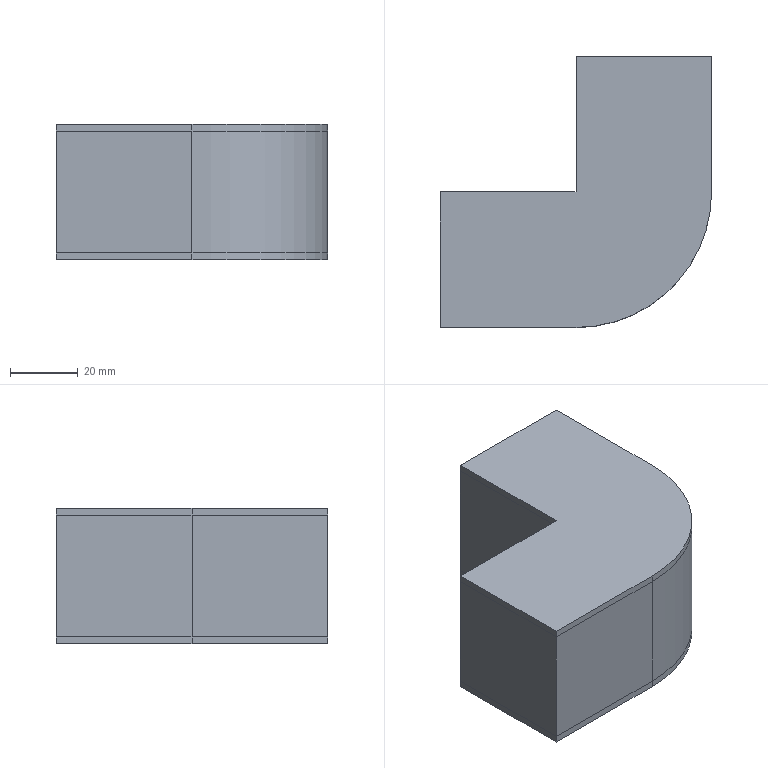Part | 3 solids | 34 faces | box 80 x 80 x 40 mm | volume 39085 mm3 | plane 30 | cylinder 4 | commonest cylinder face diameters 80 x3 76 x1
STEP:
#1=CARTESIAN_POINT('',(-40.,0.,38.));
#2=VERTEX_POINT('',#1);
#3=CARTESIAN_POINT('',(0.,0.,38.));
#4=VERTEX_POINT('',#3);
#5=CARTESIAN_POINT('',(-40.,0.,38.));
#6=DIRECTION('',(1.,0.,0.));
#7=VECTOR('',#6,1000.);
#8=LINE('',#5,#7);
#9=EDGE_CURVE('',#2,#4,#8,.T.);
#10=ORIENTED_EDGE('',*,*,#9,.F.);
#11=CARTESIAN_POINT('',(-40.,0.,40.));
#12=VERTEX_POINT('',#11);
#13=CARTESIAN_POINT('',(-40.,0.,40.));
#14=DIRECTION('',(0.,0.,-1.));
#15=VECTOR('',#14,1000.);
#16=LINE('',#13,#15);
#17=EDGE_CURVE('',#12,#2,#16,.T.);
#18=ORIENTED_EDGE('',*,*,#17,.F.);
#19=CARTESIAN_POINT('',(0.,0.,40.));
#20=VERTEX_POINT('',#19);
#21=CARTESIAN_POINT('',(-40.,0.,40.));
#22=DIRECTION('',(-1.,0.,0.));
#23=VECTOR('',#22,1000.);
#24=LINE('',#21,#23);
#25=EDGE_CURVE('',#20,#12,#24,.T.);
#26=ORIENTED_EDGE('',*,*,#25,.F.);
#27=CARTESIAN_POINT('',(0.,0.,40.));
#28=DIRECTION('',(0.,0.,-1.));
#29=VECTOR('',#28,1000.);
#30=LINE('',#27,#29);
#31=EDGE_CURVE('',#20,#4,#30,.T.);
#32=ORIENTED_EDGE('',*,*,#31,.T.);
#33=EDGE_LOOP('',(#10,#18,#26,#32));
#34=FACE_OUTER_BOUND('',#33,.T.);
#35=CARTESIAN_POINT('',(-40.,0.,40.));
#36=DIRECTION('',(0.,-1.,0.));
#37=DIRECTION('',(0.,0.,-1.));
#38=AXIS2_PLACEMENT_3D('',#35,#36,#37);
#39=PLANE('',#38);
#40=ADVANCED_FACE('',(#34),#39,.F.);
#41=CARTESIAN_POINT('',(-40.,-40.,38.));
#42=VERTEX_POINT('',#41);
#43=CARTESIAN_POINT('',(-40.,-40.,38.));
#44=DIRECTION('',(0.,1.,0.));
#45=VECTOR('',#44,1000.);
#46=LINE('',#43,#45);
#47=EDGE_CURVE('',#42,#2,#46,.T.);
#48=ORIENTED_EDGE('',*,*,#47,.F.);
#49=CARTESIAN_POINT('',(-40.,-40.,40.));
#50=VERTEX_POINT('',#49);
#51=CARTESIAN_POINT('',(-40.,-40.,40.));
#52=DIRECTION('',(0.,0.,-1.));
#53=VECTOR('',#52,1000.);
#54=LINE('',#51,#53);
#55=EDGE_CURVE('',#50,#42,#54,.T.);
#56=ORIENTED_EDGE('',*,*,#55,.F.);
#57=CARTESIAN_POINT('',(-40.,-40.,40.));
#58=DIRECTION('',(0.,-1.,0.));
#59=VECTOR('',#58,1000.);
#60=LINE('',#57,#59);
#61=EDGE_CURVE('',#12,#50,#60,.T.);
#62=ORIENTED_EDGE('',*,*,#61,.F.);
#63=ORIENTED_EDGE('',*,*,#17,.T.);
#64=EDGE_LOOP('',(#48,#56,#62,#63));
#65=FACE_OUTER_BOUND('',#64,.T.);
#66=CARTESIAN_POINT('',(-40.,-40.,40.));
#67=DIRECTION('',(1.,0.,0.));
#68=DIRECTION('',(0.,0.,-1.));
#69=AXIS2_PLACEMENT_3D('',#66,#67,#68);
#70=PLANE('',#69);
#71=ADVANCED_FACE('',(#65),#70,.F.);
#72=CARTESIAN_POINT('',(0.,-40.,38.));
#73=VERTEX_POINT('',#72);
#74=CARTESIAN_POINT('',(0.,-40.,38.));
#75=DIRECTION('',(-1.,0.,0.));
#76=VECTOR('',#75,1000.);
#77=LINE('',#74,#76);
#78=EDGE_CURVE('',#73,#42,#77,.T.);
#79=ORIENTED_EDGE('',*,*,#78,.F.);
#80=CARTESIAN_POINT('',(0.,-40.,40.));
#81=VERTEX_POINT('',#80);
#82=CARTESIAN_POINT('',(0.,-40.,40.));
#83=DIRECTION('',(0.,0.,-1.));
#84=VECTOR('',#83,1000.);
#85=LINE('',#82,#84);
#86=EDGE_CURVE('',#81,#73,#85,.T.);
#87=ORIENTED_EDGE('',*,*,#86,.F.);
#88=CARTESIAN_POINT('',(0.,-40.,40.));
#89=DIRECTION('',(1.,0.,0.));
#90=VECTOR('',#89,1000.);
#91=LINE('',#88,#90);
#92=EDGE_CURVE('',#50,#81,#91,.T.);
#93=ORIENTED_EDGE('',*,*,#92,.F.);
#94=ORIENTED_EDGE('',*,*,#55,.T.);
#95=EDGE_LOOP('',(#79,#87,#93,#94));
#96=FACE_OUTER_BOUND('',#95,.T.);
#97=CARTESIAN_POINT('',(0.,-40.,40.));
#98=DIRECTION('',(0.,1.,0.));
#99=DIRECTION('',(0.,0.,1.));
#100=AXIS2_PLACEMENT_3D('',#97,#98,#99);
#101=PLANE('',#100);
#102=ADVANCED_FACE('',(#96),#101,.F.);
#103=CARTESIAN_POINT('',(40.,0.,38.));
#104=VERTEX_POINT('',#103);
#105=CARTESIAN_POINT('',(0.,0.,38.));
#106=DIRECTION('',(0.,0.,-1.));
#107=DIRECTION('',(-1.,0.,0.));
#108=AXIS2_PLACEMENT_3D('',#105,#106,#107);
#109=CIRCLE('',#108,40.);
#110=EDGE_CURVE('',#104,#73,#109,.T.);
#111=ORIENTED_EDGE('',*,*,#110,.F.);
#112=CARTESIAN_POINT('',(40.,0.,40.));
#113=VERTEX_POINT('',#112);
#114=CARTESIAN_POINT('',(40.,0.,40.));
#115=DIRECTION('',(0.,0.,-1.));
#116=VECTOR('',#115,1000.);
#117=LINE('',#114,#116);
#118=EDGE_CURVE('',#113,#104,#117,.T.);
#119=ORIENTED_EDGE('',*,*,#118,.F.);
#120=CARTESIAN_POINT('',(0.,0.,40.));
#121=DIRECTION('',(0.,0.,1.));
#122=DIRECTION('',(1.,0.,0.));
#123=AXIS2_PLACEMENT_3D('',#120,#121,#122);
#124=CIRCLE('',#123,40.);
#125=EDGE_CURVE('',#81,#113,#124,.T.);
#126=ORIENTED_EDGE('',*,*,#125,.F.);
#127=ORIENTED_EDGE('',*,*,#86,.T.);
#128=EDGE_LOOP('',(#111,#119,#126,#127));
#129=FACE_OUTER_BOUND('',#128,.T.);
#130=CARTESIAN_POINT('',(0.,0.,40.));
#131=DIRECTION('',(0.,0.,-1.));
#132=DIRECTION('',(-1.,0.,0.));
#133=AXIS2_PLACEMENT_3D('',#130,#131,#132);
#134=CYLINDRICAL_SURFACE('',#133,40.);
#135=ADVANCED_FACE('',(#129),#134,.T.);
#136=CARTESIAN_POINT('',(40.,40.,38.));
#137=VERTEX_POINT('',#136);
#138=CARTESIAN_POINT('',(40.,0.,38.));
#139=DIRECTION('',(0.,-1.,0.));
#140=VECTOR('',#139,1000.);
#141=LINE('',#138,#140);
#142=EDGE_CURVE('',#137,#104,#141,.T.);
#143=ORIENTED_EDGE('',*,*,#142,.F.);
#144=CARTESIAN_POINT('',(40.,40.,40.));
#145=VERTEX_POINT('',#144);
#146=CARTESIAN_POINT('',(40.,40.,40.));
#147=DIRECTION('',(0.,0.,-1.));
#148=VECTOR('',#147,1000.);
#149=LINE('',#146,#148);
#150=EDGE_CURVE('',#145,#137,#149,.T.);
#151=ORIENTED_EDGE('',*,*,#150,.F.);
#152=CARTESIAN_POINT('',(40.,0.,40.));
#153=DIRECTION('',(0.,1.,0.));
#154=VECTOR('',#153,1000.);
#155=LINE('',#152,#154);
#156=EDGE_CURVE('',#113,#145,#155,.T.);
#157=ORIENTED_EDGE('',*,*,#156,.F.);
#158=ORIENTED_EDGE('',*,*,#118,.T.);
#159=EDGE_LOOP('',(#143,#151,#157,#158));
#160=FACE_OUTER_BOUND('',#159,.T.);
#161=CARTESIAN_POINT('',(40.,0.,40.));
#162=DIRECTION('',(-1.,0.,0.));
#163=DIRECTION('',(0.,0.,1.));
#164=AXIS2_PLACEMENT_3D('',#161,#162,#163);
#165=PLANE('',#164);
#166=ADVANCED_FACE('',(#160),#165,.F.);
#167=CARTESIAN_POINT('',(0.,40.,38.));
#168=VERTEX_POINT('',#167);
#169=CARTESIAN_POINT('',(0.,40.,38.));
#170=DIRECTION('',(1.,0.,0.));
#171=VECTOR('',#170,1000.);
#172=LINE('',#169,#171);
#173=EDGE_CURVE('',#168,#137,#172,.T.);
#174=ORIENTED_EDGE('',*,*,#173,.F.);
#175=CARTESIAN_POINT('',(0.,40.,40.));
#176=VERTEX_POINT('',#175);
#177=CARTESIAN_POINT('',(0.,40.,40.));
#178=DIRECTION('',(0.,0.,-1.));
#179=VECTOR('',#178,1000.);
#180=LINE('',#177,#179);
#181=EDGE_CURVE('',#176,#168,#180,.T.);
#182=ORIENTED_EDGE('',*,*,#181,.F.);
#183=CARTESIAN_POINT('',(0.,40.,40.));
#184=DIRECTION('',(-1.,0.,0.));
#185=VECTOR('',#184,1000.);
#186=LINE('',#183,#185);
#187=EDGE_CURVE('',#145,#176,#186,.T.);
#188=ORIENTED_EDGE('',*,*,#187,.F.);
#189=ORIENTED_EDGE('',*,*,#150,.T.);
#190=EDGE_LOOP('',(#174,#182,#188,#189));
#191=FACE_OUTER_BOUND('',#190,.T.);
#192=CARTESIAN_POINT('',(0.,40.,40.));
#193=DIRECTION('',(0.,-1.,0.));
#194=DIRECTION('',(0.,0.,-1.));
#195=AXIS2_PLACEMENT_3D('',#192,#193,#194);
#196=PLANE('',#195);
#197=ADVANCED_FACE('',(#191),#196,.F.);
#198=CARTESIAN_POINT('',(0.,0.,38.));
#199=DIRECTION('',(0.,1.,0.));
#200=VECTOR('',#199,1000.);
#201=LINE('',#198,#200);
#202=EDGE_CURVE('',#4,#168,#201,.T.);
#203=ORIENTED_EDGE('',*,*,#202,.F.);
#204=ORIENTED_EDGE('',*,*,#31,.F.);
#205=CARTESIAN_POINT('',(0.,0.,40.));
#206=DIRECTION('',(0.,-1.,0.));
#207=VECTOR('',#206,1000.);
#208=LINE('',#205,#207);
#209=EDGE_CURVE('',#176,#20,#208,.T.);
#210=ORIENTED_EDGE('',*,*,#209,.F.);
#211=ORIENTED_EDGE('',*,*,#181,.T.);
#212=EDGE_LOOP('',(#203,#204,#210,#211));
#213=FACE_OUTER_BOUND('',#212,.T.);
#214=CARTESIAN_POINT('',(0.,0.,40.));
#215=DIRECTION('',(1.,0.,0.));
#216=DIRECTION('',(0.,0.,-1.));
#217=AXIS2_PLACEMENT_3D('',#214,#215,#216);
#218=PLANE('',#217);
#219=ADVANCED_FACE('',(#213),#218,.F.);
#220=ORIENTED_EDGE('',*,*,#25,.T.);
#221=ORIENTED_EDGE('',*,*,#61,.T.);
#222=ORIENTED_EDGE('',*,*,#92,.T.);
#223=ORIENTED_EDGE('',*,*,#125,.T.);
#224=ORIENTED_EDGE('',*,*,#156,.T.);
#225=ORIENTED_EDGE('',*,*,#187,.T.);
#226=ORIENTED_EDGE('',*,*,#209,.T.);
#227=EDGE_LOOP('',(#220,#221,#222,#223,#224,#225,#226));
#228=FACE_OUTER_BOUND('',#227,.T.);
#229=CARTESIAN_POINT('',(0.,0.,40.));
#230=DIRECTION('',(0.,0.,1.));
#231=DIRECTION('',(1.,0.,0.));
#232=AXIS2_PLACEMENT_3D('',#229,#230,#231);
#233=PLANE('',#232);
#234=ADVANCED_FACE('',(#228),#233,.T.);
#235=ORIENTED_EDGE('',*,*,#47,.T.);
#236=ORIENTED_EDGE('',*,*,#9,.T.);
#237=ORIENTED_EDGE('',*,*,#202,.T.);
#238=ORIENTED_EDGE('',*,*,#173,.T.);
#239=ORIENTED_EDGE('',*,*,#142,.T.);
#240=ORIENTED_EDGE('',*,*,#110,.T.);
#241=ORIENTED_EDGE('',*,*,#78,.T.);
#242=EDGE_LOOP('',(#235,#236,#237,#238,#239,#240,#241));
#243=FACE_OUTER_BOUND('',#242,.T.);
#244=CARTESIAN_POINT('',(2.,38.,38.));
#245=DIRECTION('',(0.,0.,-1.));
#246=DIRECTION('',(-1.,0.,0.));
#247=AXIS2_PLACEMENT_3D('',#244,#245,#246);
#248=PLANE('',#247);
#249=ADVANCED_FACE('',(#243),#248,.T.);
#250=CLOSED_SHELL('',(#40,#71,#102,#135,#166,#197,#219,#234,#249));
#251=MANIFOLD_SOLID_BREP('',#250);
#252=CARTESIAN_POINT('',(-40.,-40.,2.));
#253=VERTEX_POINT('',#252);
#254=CARTESIAN_POINT('',(0.,-40.,2.));
#255=VERTEX_POINT('',#254);
#256=CARTESIAN_POINT('',(0.,-40.,2.));
#257=DIRECTION('',(1.,0.,0.));
#258=VECTOR('',#257,1000.);
#259=LINE('',#256,#258);
#260=EDGE_CURVE('',#253,#255,#259,.T.);
#261=ORIENTED_EDGE('',*,*,#260,.F.);
#262=CARTESIAN_POINT('',(-40.,-40.,0.));
#263=VERTEX_POINT('',#262);
#264=CARTESIAN_POINT('',(-40.,-40.,40.));
#265=DIRECTION('',(0.,0.,-1.));
#266=VECTOR('',#265,1000.);
#267=LINE('',#264,#266);
#268=EDGE_CURVE('',#253,#263,#267,.T.);
#269=ORIENTED_EDGE('',*,*,#268,.T.);
#270=CARTESIAN_POINT('',(0.,-40.,0.));
#271=VERTEX_POINT('',#270);
#272=CARTESIAN_POINT('',(0.,-40.,0.));
#273=DIRECTION('',(1.,0.,0.));
#274=VECTOR('',#273,1000.);
#275=LINE('',#272,#274);
#276=EDGE_CURVE('',#263,#271,#275,.T.);
#277=ORIENTED_EDGE('',*,*,#276,.T.);
#278=CARTESIAN_POINT('',(0.,-40.,40.));
#279=DIRECTION('',(0.,0.,-1.));
#280=VECTOR('',#279,1000.);
#281=LINE('',#278,#280);
#282=EDGE_CURVE('',#255,#271,#281,.T.);
#283=ORIENTED_EDGE('',*,*,#282,.F.);
#284=EDGE_LOOP('',(#261,#269,#277,#283));
#285=FACE_OUTER_BOUND('',#284,.T.);
#286=CARTESIAN_POINT('',(0.,-40.,40.));
#287=DIRECTION('',(0.,1.,0.));
#288=DIRECTION('',(0.,0.,1.));
#289=AXIS2_PLACEMENT_3D('',#286,#287,#288);
#290=PLANE('',#289);
#291=ADVANCED_FACE('',(#285),#290,.F.);
#292=CARTESIAN_POINT('',(40.,0.,2.));
#293=VERTEX_POINT('',#292);
#294=CARTESIAN_POINT('',(0.,0.,2.));
#295=DIRECTION('',(0.,0.,1.));
#296=DIRECTION('',(1.,0.,0.));
#297=AXIS2_PLACEMENT_3D('',#294,#295,#296);
#298=CIRCLE('',#297,40.);
#299=EDGE_CURVE('',#255,#293,#298,.T.);
#300=ORIENTED_EDGE('',*,*,#299,.F.);
#301=ORIENTED_EDGE('',*,*,#282,.T.);
#302=CARTESIAN_POINT('',(40.,0.,0.));
#303=VERTEX_POINT('',#302);
#304=CARTESIAN_POINT('',(0.,0.,0.));
#305=DIRECTION('',(0.,0.,1.));
#306=DIRECTION('',(1.,0.,0.));
#307=AXIS2_PLACEMENT_3D('',#304,#305,#306);
#308=CIRCLE('',#307,40.);
#309=EDGE_CURVE('',#271,#303,#308,.T.);
#310=ORIENTED_EDGE('',*,*,#309,.T.);
#311=CARTESIAN_POINT('',(40.,0.,40.));
#312=DIRECTION('',(0.,0.,-1.));
#313=VECTOR('',#312,1000.);
#314=LINE('',#311,#313);
#315=EDGE_CURVE('',#293,#303,#314,.T.);
#316=ORIENTED_EDGE('',*,*,#315,.F.);
#317=EDGE_LOOP('',(#300,#301,#310,#316));
#318=FACE_OUTER_BOUND('',#317,.T.);
#319=CARTESIAN_POINT('',(0.,0.,40.));
#320=DIRECTION('',(0.,0.,-1.));
#321=DIRECTION('',(-1.,0.,0.));
#322=AXIS2_PLACEMENT_3D('',#319,#320,#321);
#323=CYLINDRICAL_SURFACE('',#322,40.);
#324=ADVANCED_FACE('',(#318),#323,.T.);
#325=CARTESIAN_POINT('',(40.,40.,2.));
#326=VERTEX_POINT('',#325);
#327=CARTESIAN_POINT('',(40.,0.,2.));
#328=DIRECTION('',(0.,1.,0.));
#329=VECTOR('',#328,1000.);
#330=LINE('',#327,#329);
#331=EDGE_CURVE('',#293,#326,#330,.T.);
#332=ORIENTED_EDGE('',*,*,#331,.F.);
#333=ORIENTED_EDGE('',*,*,#315,.T.);
#334=CARTESIAN_POINT('',(40.,40.,0.));
#335=VERTEX_POINT('',#334);
#336=CARTESIAN_POINT('',(40.,0.,0.));
#337=DIRECTION('',(0.,1.,0.));
#338=VECTOR('',#337,1000.);
#339=LINE('',#336,#338);
#340=EDGE_CURVE('',#303,#335,#339,.T.);
#341=ORIENTED_EDGE('',*,*,#340,.T.);
#342=CARTESIAN_POINT('',(40.,40.,40.));
#343=DIRECTION('',(0.,0.,-1.));
#344=VECTOR('',#343,1000.);
#345=LINE('',#342,#344);
#346=EDGE_CURVE('',#326,#335,#345,.T.);
#347=ORIENTED_EDGE('',*,*,#346,.F.);
#348=EDGE_LOOP('',(#332,#333,#341,#347));
#349=FACE_OUTER_BOUND('',#348,.T.);
#350=CARTESIAN_POINT('',(40.,0.,40.));
#351=DIRECTION('',(-1.,0.,0.));
#352=DIRECTION('',(0.,0.,1.));
#353=AXIS2_PLACEMENT_3D('',#350,#351,#352);
#354=PLANE('',#353);
#355=ADVANCED_FACE('',(#349),#354,.F.);
#356=CARTESIAN_POINT('',(-40.,0.,2.));
#357=VERTEX_POINT('',#356);
#358=CARTESIAN_POINT('',(-40.,-40.,2.));
#359=DIRECTION('',(0.,-1.,0.));
#360=VECTOR('',#359,1000.);
#361=LINE('',#358,#360);
#362=EDGE_CURVE('',#357,#253,#361,.T.);
#363=ORIENTED_EDGE('',*,*,#362,.F.);
#364=CARTESIAN_POINT('',(-40.,0.,0.));
#365=VERTEX_POINT('',#364);
#366=CARTESIAN_POINT('',(-40.,0.,40.));
#367=DIRECTION('',(0.,0.,-1.));
#368=VECTOR('',#367,1000.);
#369=LINE('',#366,#368);
#370=EDGE_CURVE('',#357,#365,#369,.T.);
#371=ORIENTED_EDGE('',*,*,#370,.T.);
#372=CARTESIAN_POINT('',(-40.,-40.,0.));
#373=DIRECTION('',(0.,-1.,0.));
#374=VECTOR('',#373,1000.);
#375=LINE('',#372,#374);
#376=EDGE_CURVE('',#365,#263,#375,.T.);
#377=ORIENTED_EDGE('',*,*,#376,.T.);
#378=ORIENTED_EDGE('',*,*,#268,.F.);
#379=EDGE_LOOP('',(#363,#371,#377,#378));
#380=FACE_OUTER_BOUND('',#379,.T.);
#381=CARTESIAN_POINT('',(-40.,-40.,40.));
#382=DIRECTION('',(1.,0.,0.));
#383=DIRECTION('',(0.,0.,-1.));
#384=AXIS2_PLACEMENT_3D('',#381,#382,#383);
#385=PLANE('',#384);
#386=ADVANCED_FACE('',(#380),#385,.F.);
#387=CARTESIAN_POINT('',(0.,0.,2.));
#388=VERTEX_POINT('',#387);
#389=CARTESIAN_POINT('',(-40.,0.,2.));
#390=DIRECTION('',(-1.,0.,0.));
#391=VECTOR('',#390,1000.);
#392=LINE('',#389,#391);
#393=EDGE_CURVE('',#388,#357,#392,.T.);
#394=ORIENTED_EDGE('',*,*,#393,.F.);
#395=CARTESIAN_POINT('',(0.,0.,0.));
#396=VERTEX_POINT('',#395);
#397=CARTESIAN_POINT('',(0.,0.,40.));
#398=DIRECTION('',(0.,0.,-1.));
#399=VECTOR('',#398,1000.);
#400=LINE('',#397,#399);
#401=EDGE_CURVE('',#388,#396,#400,.T.);
#402=ORIENTED_EDGE('',*,*,#401,.T.);
#403=CARTESIAN_POINT('',(-40.,0.,0.));
#404=DIRECTION('',(-1.,0.,0.));
#405=VECTOR('',#404,1000.);
#406=LINE('',#403,#405);
#407=EDGE_CURVE('',#396,#365,#406,.T.);
#408=ORIENTED_EDGE('',*,*,#407,.T.);
#409=ORIENTED_EDGE('',*,*,#370,.F.);
#410=EDGE_LOOP('',(#394,#402,#408,#409));
#411=FACE_OUTER_BOUND('',#410,.T.);
#412=CARTESIAN_POINT('',(-40.,0.,40.));
#413=DIRECTION('',(0.,-1.,0.));
#414=DIRECTION('',(0.,0.,-1.));
#415=AXIS2_PLACEMENT_3D('',#412,#413,#414);
#416=PLANE('',#415);
#417=ADVANCED_FACE('',(#411),#416,.F.);
#418=ORIENTED_EDGE('',*,*,#407,.F.);
#419=CARTESIAN_POINT('',(0.,40.,0.));
#420=VERTEX_POINT('',#419);
#421=CARTESIAN_POINT('',(0.,0.,0.));
#422=DIRECTION('',(0.,-1.,0.));
#423=VECTOR('',#422,1000.);
#424=LINE('',#421,#423);
#425=EDGE_CURVE('',#420,#396,#424,.T.);
#426=ORIENTED_EDGE('',*,*,#425,.F.);
#427=CARTESIAN_POINT('',(0.,40.,0.));
#428=DIRECTION('',(-1.,0.,0.));
#429=VECTOR('',#428,1000.);
#430=LINE('',#427,#429);
#431=EDGE_CURVE('',#335,#420,#430,.T.);
#432=ORIENTED_EDGE('',*,*,#431,.F.);
#433=ORIENTED_EDGE('',*,*,#340,.F.);
#434=ORIENTED_EDGE('',*,*,#309,.F.);
#435=ORIENTED_EDGE('',*,*,#276,.F.);
#436=ORIENTED_EDGE('',*,*,#376,.F.);
#437=EDGE_LOOP('',(#418,#426,#432,#433,#434,#435,#436));
#438=FACE_OUTER_BOUND('',#437,.T.);
#439=CARTESIAN_POINT('',(0.,0.,0.));
#440=DIRECTION('',(0.,0.,1.));
#441=DIRECTION('',(1.,0.,0.));
#442=AXIS2_PLACEMENT_3D('',#439,#440,#441);
#443=PLANE('',#442);
#444=ADVANCED_FACE('',(#438),#443,.F.);
#445=CARTESIAN_POINT('',(0.,40.,2.));
#446=VERTEX_POINT('',#445);
#447=CARTESIAN_POINT('',(0.,40.,2.));
#448=DIRECTION('',(-1.,0.,0.));
#449=VECTOR('',#448,1000.);
#450=LINE('',#447,#449);
#451=EDGE_CURVE('',#326,#446,#450,.T.);
#452=ORIENTED_EDGE('',*,*,#451,.F.);
#453=ORIENTED_EDGE('',*,*,#346,.T.);
#454=ORIENTED_EDGE('',*,*,#431,.T.);
#455=CARTESIAN_POINT('',(0.,40.,40.));
#456=DIRECTION('',(0.,0.,-1.));
#457=VECTOR('',#456,1000.);
#458=LINE('',#455,#457);
#459=EDGE_CURVE('',#446,#420,#458,.T.);
#460=ORIENTED_EDGE('',*,*,#459,.F.);
#461=EDGE_LOOP('',(#452,#453,#454,#460));
#462=FACE_OUTER_BOUND('',#461,.T.);
#463=CARTESIAN_POINT('',(0.,40.,40.));
#464=DIRECTION('',(0.,-1.,0.));
#465=DIRECTION('',(0.,0.,-1.));
#466=AXIS2_PLACEMENT_3D('',#463,#464,#465);
#467=PLANE('',#466);
#468=ADVANCED_FACE('',(#462),#467,.F.);
#469=CARTESIAN_POINT('',(0.,0.,2.));
#470=DIRECTION('',(0.,-1.,0.));
#471=VECTOR('',#470,1000.);
#472=LINE('',#469,#471);
#473=EDGE_CURVE('',#446,#388,#472,.T.);
#474=ORIENTED_EDGE('',*,*,#473,.F.);
#475=ORIENTED_EDGE('',*,*,#459,.T.);
#476=ORIENTED_EDGE('',*,*,#425,.T.);
#477=ORIENTED_EDGE('',*,*,#401,.F.);
#478=EDGE_LOOP('',(#474,#475,#476,#477));
#479=FACE_OUTER_BOUND('',#478,.T.);
#480=CARTESIAN_POINT('',(0.,0.,40.));
#481=DIRECTION('',(1.,0.,0.));
#482=DIRECTION('',(0.,0.,-1.));
#483=AXIS2_PLACEMENT_3D('',#480,#481,#482);
#484=PLANE('',#483);
#485=ADVANCED_FACE('',(#479),#484,.F.);
#486=ORIENTED_EDGE('',*,*,#393,.T.);
#487=ORIENTED_EDGE('',*,*,#362,.T.);
#488=ORIENTED_EDGE('',*,*,#260,.T.);
#489=ORIENTED_EDGE('',*,*,#299,.T.);
#490=ORIENTED_EDGE('',*,*,#331,.T.);
#491=ORIENTED_EDGE('',*,*,#451,.T.);
#492=ORIENTED_EDGE('',*,*,#473,.T.);
#493=EDGE_LOOP('',(#486,#487,#488,#489,#490,#491,#492));
#494=FACE_OUTER_BOUND('',#493,.T.);
#495=CARTESIAN_POINT('',(-38.,-2.,2.));
#496=DIRECTION('',(0.,0.,1.));
#497=DIRECTION('',(1.,0.,0.));
#498=AXIS2_PLACEMENT_3D('',#495,#496,#497);
#499=PLANE('',#498);
#500=ADVANCED_FACE('',(#494),#499,.T.);
#501=CLOSED_SHELL('',(#291,#324,#355,#386,#417,#444,#468,#485,#500));
#502=MANIFOLD_SOLID_BREP('',#501);
#503=CARTESIAN_POINT('',(0.,-38.,2.));
#504=VERTEX_POINT('',#503);
#505=CARTESIAN_POINT('',(38.,0.,2.));
#506=VERTEX_POINT('',#505);
#507=CARTESIAN_POINT('',(0.,0.,2.));
#508=DIRECTION('',(0.,0.,1.));
#509=DIRECTION('',(1.,0.,0.));
#510=AXIS2_PLACEMENT_3D('',#507,#508,#509);
#511=CIRCLE('',#510,38.);
#512=EDGE_CURVE('',#504,#506,#511,.T.);
#513=ORIENTED_EDGE('',*,*,#512,.T.);
#514=CARTESIAN_POINT('',(38.,38.,2.));
#515=VERTEX_POINT('',#514);
#516=CARTESIAN_POINT('',(38.,0.,2.));
#517=DIRECTION('',(0.,1.,0.));
#518=VECTOR('',#517,1000.);
#519=LINE('',#516,#518);
#520=EDGE_CURVE('',#506,#515,#519,.T.);
#521=ORIENTED_EDGE('',*,*,#520,.T.);
#522=CARTESIAN_POINT('',(2.,38.,2.));
#523=VERTEX_POINT('',#522);
#524=CARTESIAN_POINT('',(0.,38.,2.));
#525=DIRECTION('',(-1.,0.,0.));
#526=VECTOR('',#525,1000.);
#527=LINE('',#524,#526);
#528=EDGE_CURVE('',#515,#523,#527,.T.);
#529=ORIENTED_EDGE('',*,*,#528,.T.);
#530=CARTESIAN_POINT('',(2.,-2.,2.));
#531=VERTEX_POINT('',#530);
#532=CARTESIAN_POINT('',(2.,0.,2.));
#533=DIRECTION('',(0.,-1.,0.));
#534=VECTOR('',#533,1000.);
#535=LINE('',#532,#534);
#536=EDGE_CURVE('',#523,#531,#535,.T.);
#537=ORIENTED_EDGE('',*,*,#536,.T.);
#538=CARTESIAN_POINT('',(-38.,-2.,2.));
#539=VERTEX_POINT('',#538);
#540=CARTESIAN_POINT('',(-40.,-2.,2.));
#541=DIRECTION('',(-1.,0.,0.));
#542=VECTOR('',#541,1000.);
#543=LINE('',#540,#542);
#544=EDGE_CURVE('',#531,#539,#543,.T.);
#545=ORIENTED_EDGE('',*,*,#544,.T.);
#546=CARTESIAN_POINT('',(-38.,-38.,2.));
#547=VERTEX_POINT('',#546);
#548=CARTESIAN_POINT('',(-38.,-40.,2.));
#549=DIRECTION('',(0.,-1.,0.));
#550=VECTOR('',#549,1000.);
#551=LINE('',#548,#550);
#552=EDGE_CURVE('',#539,#547,#551,.T.);
#553=ORIENTED_EDGE('',*,*,#552,.T.);
#554=CARTESIAN_POINT('',(0.,-38.,2.));
#555=DIRECTION('',(1.,0.,0.));
#556=VECTOR('',#555,1000.);
#557=LINE('',#554,#556);
#558=EDGE_CURVE('',#547,#504,#557,.T.);
#559=ORIENTED_EDGE('',*,*,#558,.T.);
#560=EDGE_LOOP('',(#513,#521,#529,#537,#545,#553,#559));
#561=FACE_BOUND('',#560,.T.);
#562=CARTESIAN_POINT('',(0.,0.,2.));
#563=VERTEX_POINT('',#562);
#564=CARTESIAN_POINT('',(-40.,0.,2.));
#565=VERTEX_POINT('',#564);
#566=CARTESIAN_POINT('',(-40.,0.,2.));
#567=DIRECTION('',(-1.,0.,0.));
#568=VECTOR('',#567,1000.);
#569=LINE('',#566,#568);
#570=EDGE_CURVE('',#563,#565,#569,.T.);
#571=ORIENTED_EDGE('',*,*,#570,.F.);
#572=CARTESIAN_POINT('',(0.,40.,2.));
#573=VERTEX_POINT('',#572);
#574=CARTESIAN_POINT('',(0.,0.,2.));
#575=DIRECTION('',(0.,-1.,0.));
#576=VECTOR('',#575,1000.);
#577=LINE('',#574,#576);
#578=EDGE_CURVE('',#573,#563,#577,.T.);
#579=ORIENTED_EDGE('',*,*,#578,.F.);
#580=CARTESIAN_POINT('',(40.,40.,2.));
#581=VERTEX_POINT('',#580);
#582=CARTESIAN_POINT('',(0.,40.,2.));
#583=DIRECTION('',(-1.,0.,0.));
#584=VECTOR('',#583,1000.);
#585=LINE('',#582,#584);
#586=EDGE_CURVE('',#581,#573,#585,.T.);
#587=ORIENTED_EDGE('',*,*,#586,.F.);
#588=CARTESIAN_POINT('',(40.,0.,2.));
#589=VERTEX_POINT('',#588);
#590=CARTESIAN_POINT('',(40.,0.,2.));
#591=DIRECTION('',(0.,1.,0.));
#592=VECTOR('',#591,1000.);
#593=LINE('',#590,#592);
#594=EDGE_CURVE('',#589,#581,#593,.T.);
#595=ORIENTED_EDGE('',*,*,#594,.F.);
#596=CARTESIAN_POINT('',(0.,-40.,2.));
#597=VERTEX_POINT('',#596);
#598=CARTESIAN_POINT('',(0.,0.,2.));
#599=DIRECTION('',(0.,0.,1.));
#600=DIRECTION('',(1.,0.,0.));
#601=AXIS2_PLACEMENT_3D('',#598,#599,#600);
#602=CIRCLE('',#601,40.);
#603=EDGE_CURVE('',#597,#589,#602,.T.);
#604=ORIENTED_EDGE('',*,*,#603,.F.);
#605=CARTESIAN_POINT('',(-40.,-40.,2.));
#606=VERTEX_POINT('',#605);
#607=CARTESIAN_POINT('',(0.,-40.,2.));
#608=DIRECTION('',(1.,0.,0.));
#609=VECTOR('',#608,1000.);
#610=LINE('',#607,#609);
#611=EDGE_CURVE('',#606,#597,#610,.T.);
#612=ORIENTED_EDGE('',*,*,#611,.F.);
#613=CARTESIAN_POINT('',(-40.,-40.,2.));
#614=DIRECTION('',(0.,-1.,0.));
#615=VECTOR('',#614,1000.);
#616=LINE('',#613,#615);
#617=EDGE_CURVE('',#565,#606,#616,.T.);
#618=ORIENTED_EDGE('',*,*,#617,.F.);
#619=EDGE_LOOP('',(#571,#579,#587,#595,#604,#612,#618));
#620=FACE_OUTER_BOUND('',#619,.T.);
#621=CARTESIAN_POINT('',(-38.,-2.,2.));
#622=DIRECTION('',(0.,0.,1.));
#623=DIRECTION('',(1.,0.,0.));
#624=AXIS2_PLACEMENT_3D('',#621,#622,#623);
#625=PLANE('',#624);
#626=ADVANCED_FACE('',(#561,#620),#625,.F.);
#627=CARTESIAN_POINT('',(2.,-2.,38.));
#628=VERTEX_POINT('',#627);
#629=CARTESIAN_POINT('',(2.,-2.,40.));
#630=DIRECTION('',(0.,0.,-1.));
#631=VECTOR('',#630,1000.);
#632=LINE('',#629,#631);
#633=EDGE_CURVE('',#628,#531,#632,.T.);
#634=ORIENTED_EDGE('',*,*,#633,.F.);
#635=CARTESIAN_POINT('',(-38.,-2.,38.));
#636=VERTEX_POINT('',#635);
#637=CARTESIAN_POINT('',(2.,-2.,38.));
#638=DIRECTION('',(-1.,0.,0.));
#639=VECTOR('',#638,1000.);
#640=LINE('',#637,#639);
#641=EDGE_CURVE('',#628,#636,#640,.T.);
#642=ORIENTED_EDGE('',*,*,#641,.T.);
#643=CARTESIAN_POINT('',(-38.,-2.,40.));
#644=DIRECTION('',(0.,0.,-1.));
#645=VECTOR('',#644,1000.);
#646=LINE('',#643,#645);
#647=EDGE_CURVE('',#636,#539,#646,.T.);
#648=ORIENTED_EDGE('',*,*,#647,.T.);
#649=ORIENTED_EDGE('',*,*,#544,.F.);
#650=EDGE_LOOP('',(#634,#642,#648,#649));
#651=FACE_OUTER_BOUND('',#650,.T.);
#652=CARTESIAN_POINT('',(-40.,-2.,40.));
#653=DIRECTION('',(0.,-1.,0.));
#654=DIRECTION('',(0.,0.,-1.));
#655=AXIS2_PLACEMENT_3D('',#652,#653,#654);
#656=PLANE('',#655);
#657=ADVANCED_FACE('',(#651),#656,.T.);
#658=CARTESIAN_POINT('',(2.,38.,38.));
#659=VERTEX_POINT('',#658);
#660=CARTESIAN_POINT('',(2.,38.,40.));
#661=DIRECTION('',(0.,0.,-1.));
#662=VECTOR('',#661,1000.);
#663=LINE('',#660,#662);
#664=EDGE_CURVE('',#659,#523,#663,.T.);
#665=ORIENTED_EDGE('',*,*,#664,.F.);
#666=CARTESIAN_POINT('',(2.,38.,38.));
#667=DIRECTION('',(0.,-1.,0.));
#668=VECTOR('',#667,1000.);
#669=LINE('',#666,#668);
#670=EDGE_CURVE('',#659,#628,#669,.T.);
#671=ORIENTED_EDGE('',*,*,#670,.T.);
#672=ORIENTED_EDGE('',*,*,#633,.T.);
#673=ORIENTED_EDGE('',*,*,#536,.F.);
#674=EDGE_LOOP('',(#665,#671,#672,#673));
#675=FACE_OUTER_BOUND('',#674,.T.);
#676=CARTESIAN_POINT('',(2.,0.,40.));
#677=DIRECTION('',(1.,0.,0.));
#678=DIRECTION('',(0.,0.,-1.));
#679=AXIS2_PLACEMENT_3D('',#676,#677,#678);
#680=PLANE('',#679);
#681=ADVANCED_FACE('',(#675),#680,.T.);
#682=CARTESIAN_POINT('',(0.,40.,38.));
#683=VERTEX_POINT('',#682);
#684=CARTESIAN_POINT('',(0.,40.,40.));
#685=DIRECTION('',(0.,0.,-1.));
#686=VECTOR('',#685,1000.);
#687=LINE('',#684,#686);
#688=EDGE_CURVE('',#683,#573,#687,.T.);
#689=ORIENTED_EDGE('',*,*,#688,.T.);
#690=ORIENTED_EDGE('',*,*,#578,.T.);
#691=CARTESIAN_POINT('',(0.,0.,38.));
#692=VERTEX_POINT('',#691);
#693=CARTESIAN_POINT('',(0.,0.,40.));
#694=DIRECTION('',(0.,0.,-1.));
#695=VECTOR('',#694,1000.);
#696=LINE('',#693,#695);
#697=EDGE_CURVE('',#692,#563,#696,.T.);
#698=ORIENTED_EDGE('',*,*,#697,.F.);
#699=CARTESIAN_POINT('',(0.,0.,38.));
#700=DIRECTION('',(0.,1.,0.));
#701=VECTOR('',#700,1000.);
#702=LINE('',#699,#701);
#703=EDGE_CURVE('',#692,#683,#702,.T.);
#704=ORIENTED_EDGE('',*,*,#703,.T.);
#705=EDGE_LOOP('',(#689,#690,#698,#704));
#706=FACE_OUTER_BOUND('',#705,.T.);
#707=CARTESIAN_POINT('',(0.,0.,40.));
#708=DIRECTION('',(1.,0.,0.));
#709=DIRECTION('',(0.,0.,-1.));
#710=AXIS2_PLACEMENT_3D('',#707,#708,#709);
#711=PLANE('',#710);
#712=ADVANCED_FACE('',(#706),#711,.F.);
#713=CARTESIAN_POINT('',(40.,40.,38.));
#714=VERTEX_POINT('',#713);
#715=CARTESIAN_POINT('',(40.,40.,40.));
#716=DIRECTION('',(0.,0.,-1.));
#717=VECTOR('',#716,1000.);
#718=LINE('',#715,#717);
#719=EDGE_CURVE('',#714,#581,#718,.T.);
#720=ORIENTED_EDGE('',*,*,#719,.T.);
#721=ORIENTED_EDGE('',*,*,#586,.T.);
#722=ORIENTED_EDGE('',*,*,#688,.F.);
#723=CARTESIAN_POINT('',(0.,40.,38.));
#724=DIRECTION('',(1.,0.,0.));
#725=VECTOR('',#724,1000.);
#726=LINE('',#723,#725);
#727=EDGE_CURVE('',#683,#714,#726,.T.);
#728=ORIENTED_EDGE('',*,*,#727,.T.);
#729=EDGE_LOOP('',(#720,#721,#722,#728));
#730=FACE_OUTER_BOUND('',#729,.T.);
#731=CARTESIAN_POINT('',(0.,40.,40.));
#732=DIRECTION('',(0.,-1.,0.));
#733=DIRECTION('',(0.,0.,-1.));
#734=AXIS2_PLACEMENT_3D('',#731,#732,#733);
#735=PLANE('',#734);
#736=ADVANCED_FACE('',(#730),#735,.F.);
#737=ORIENTED_EDGE('',*,*,#697,.T.);
#738=ORIENTED_EDGE('',*,*,#570,.T.);
#739=CARTESIAN_POINT('',(-40.,0.,38.));
#740=VERTEX_POINT('',#739);
#741=CARTESIAN_POINT('',(-40.,0.,40.));
#742=DIRECTION('',(0.,0.,-1.));
#743=VECTOR('',#742,1000.);
#744=LINE('',#741,#743);
#745=EDGE_CURVE('',#740,#565,#744,.T.);
#746=ORIENTED_EDGE('',*,*,#745,.F.);
#747=CARTESIAN_POINT('',(-40.,0.,38.));
#748=DIRECTION('',(1.,0.,0.));
#749=VECTOR('',#748,1000.);
#750=LINE('',#747,#749);
#751=EDGE_CURVE('',#740,#692,#750,.T.);
#752=ORIENTED_EDGE('',*,*,#751,.T.);
#753=EDGE_LOOP('',(#737,#738,#746,#752));
#754=FACE_OUTER_BOUND('',#753,.T.);
#755=CARTESIAN_POINT('',(-40.,0.,40.));
#756=DIRECTION('',(0.,-1.,0.));
#757=DIRECTION('',(0.,0.,-1.));
#758=AXIS2_PLACEMENT_3D('',#755,#756,#757);
#759=PLANE('',#758);
#760=ADVANCED_FACE('',(#754),#759,.F.);
#761=CARTESIAN_POINT('',(38.,38.,38.));
#762=VERTEX_POINT('',#761);
#763=CARTESIAN_POINT('',(38.,38.,38.));
#764=DIRECTION('',(-1.,0.,0.));
#765=VECTOR('',#764,1000.);
#766=LINE('',#763,#765);
#767=EDGE_CURVE('',#762,#659,#766,.T.);
#768=ORIENTED_EDGE('',*,*,#767,.F.);
#769=CARTESIAN_POINT('',(38.,0.,38.));
#770=VERTEX_POINT('',#769);
#771=CARTESIAN_POINT('',(38.,0.,38.));
#772=DIRECTION('',(0.,1.,0.));
#773=VECTOR('',#772,1000.);
#774=LINE('',#771,#773);
#775=EDGE_CURVE('',#770,#762,#774,.T.);
#776=ORIENTED_EDGE('',*,*,#775,.F.);
#777=CARTESIAN_POINT('',(0.,-38.,38.));
#778=VERTEX_POINT('',#777);
#779=CARTESIAN_POINT('',(0.,0.,38.));
#780=DIRECTION('',(0.,0.,1.));
#781=DIRECTION('',(1.,0.,0.));
#782=AXIS2_PLACEMENT_3D('',#779,#780,#781);
#783=CIRCLE('',#782,38.);
#784=EDGE_CURVE('',#778,#770,#783,.T.);
#785=ORIENTED_EDGE('',*,*,#784,.F.);
#786=CARTESIAN_POINT('',(-38.,-38.,38.));
#787=VERTEX_POINT('',#786);
#788=CARTESIAN_POINT('',(-38.,-38.,38.));
#789=DIRECTION('',(1.,0.,0.));
#790=VECTOR('',#789,1000.);
#791=LINE('',#788,#790);
#792=EDGE_CURVE('',#787,#778,#791,.T.);
#793=ORIENTED_EDGE('',*,*,#792,.F.);
#794=CARTESIAN_POINT('',(-38.,-2.,38.));
#795=DIRECTION('',(0.,-1.,0.));
#796=VECTOR('',#795,1000.);
#797=LINE('',#794,#796);
#798=EDGE_CURVE('',#636,#787,#797,.T.);
#799=ORIENTED_EDGE('',*,*,#798,.F.);
#800=ORIENTED_EDGE('',*,*,#641,.F.);
#801=ORIENTED_EDGE('',*,*,#670,.F.);
#802=EDGE_LOOP('',(#768,#776,#785,#793,#799,#800,#801));
#803=FACE_BOUND('',#802,.T.);
#804=CARTESIAN_POINT('',(-40.,-40.,38.));
#805=VERTEX_POINT('',#804);
#806=CARTESIAN_POINT('',(-40.,-40.,38.));
#807=DIRECTION('',(0.,1.,0.));
#808=VECTOR('',#807,1000.);
#809=LINE('',#806,#808);
#810=EDGE_CURVE('',#805,#740,#809,.T.);
#811=ORIENTED_EDGE('',*,*,#810,.F.);
#812=CARTESIAN_POINT('',(0.,-40.,38.));
#813=VERTEX_POINT('',#812);
#814=CARTESIAN_POINT('',(0.,-40.,38.));
#815=DIRECTION('',(-1.,0.,0.));
#816=VECTOR('',#815,1000.);
#817=LINE('',#814,#816);
#818=EDGE_CURVE('',#813,#805,#817,.T.);
#819=ORIENTED_EDGE('',*,*,#818,.F.);
#820=CARTESIAN_POINT('',(40.,0.,38.));
#821=VERTEX_POINT('',#820);
#822=CARTESIAN_POINT('',(0.,0.,38.));
#823=DIRECTION('',(0.,0.,-1.));
#824=DIRECTION('',(-1.,0.,0.));
#825=AXIS2_PLACEMENT_3D('',#822,#823,#824);
#826=CIRCLE('',#825,40.);
#827=EDGE_CURVE('',#821,#813,#826,.T.);
#828=ORIENTED_EDGE('',*,*,#827,.F.);
#829=CARTESIAN_POINT('',(40.,0.,38.));
#830=DIRECTION('',(0.,-1.,0.));
#831=VECTOR('',#830,1000.);
#832=LINE('',#829,#831);
#833=EDGE_CURVE('',#714,#821,#832,.T.);
#834=ORIENTED_EDGE('',*,*,#833,.F.);
#835=ORIENTED_EDGE('',*,*,#727,.F.);
#836=ORIENTED_EDGE('',*,*,#703,.F.);
#837=ORIENTED_EDGE('',*,*,#751,.F.);
#838=EDGE_LOOP('',(#811,#819,#828,#834,#835,#836,#837));
#839=FACE_OUTER_BOUND('',#838,.T.);
#840=CARTESIAN_POINT('',(2.,38.,38.));
#841=DIRECTION('',(0.,0.,-1.));
#842=DIRECTION('',(-1.,0.,0.));
#843=AXIS2_PLACEMENT_3D('',#840,#841,#842);
#844=PLANE('',#843);
#845=ADVANCED_FACE('',(#803,#839),#844,.F.);
#846=ORIENTED_EDGE('',*,*,#745,.T.);
#847=ORIENTED_EDGE('',*,*,#617,.T.);
#848=CARTESIAN_POINT('',(-40.,-40.,40.));
#849=DIRECTION('',(0.,0.,-1.));
#850=VECTOR('',#849,1000.);
#851=LINE('',#848,#850);
#852=EDGE_CURVE('',#805,#606,#851,.T.);
#853=ORIENTED_EDGE('',*,*,#852,.F.);
#854=ORIENTED_EDGE('',*,*,#810,.T.);
#855=EDGE_LOOP('',(#846,#847,#853,#854));
#856=FACE_OUTER_BOUND('',#855,.T.);
#857=CARTESIAN_POINT('',(-40.,-40.,40.));
#858=DIRECTION('',(1.,0.,0.));
#859=DIRECTION('',(0.,0.,-1.));
#860=AXIS2_PLACEMENT_3D('',#857,#858,#859);
#861=PLANE('',#860);
#862=ADVANCED_FACE('',(#856),#861,.F.);
#863=CARTESIAN_POINT('',(40.,0.,40.));
#864=DIRECTION('',(0.,0.,-1.));
#865=VECTOR('',#864,1000.);
#866=LINE('',#863,#865);
#867=EDGE_CURVE('',#821,#589,#866,.T.);
#868=ORIENTED_EDGE('',*,*,#867,.T.);
#869=ORIENTED_EDGE('',*,*,#594,.T.);
#870=ORIENTED_EDGE('',*,*,#719,.F.);
#871=ORIENTED_EDGE('',*,*,#833,.T.);
#872=EDGE_LOOP('',(#868,#869,#870,#871));
#873=FACE_OUTER_BOUND('',#872,.T.);
#874=CARTESIAN_POINT('',(40.,0.,40.));
#875=DIRECTION('',(-1.,0.,0.));
#876=DIRECTION('',(0.,0.,1.));
#877=AXIS2_PLACEMENT_3D('',#874,#875,#876);
#878=PLANE('',#877);
#879=ADVANCED_FACE('',(#873),#878,.F.);
#880=CARTESIAN_POINT('',(0.,-40.,40.));
#881=DIRECTION('',(0.,0.,-1.));
#882=VECTOR('',#881,1000.);
#883=LINE('',#880,#882);
#884=EDGE_CURVE('',#813,#597,#883,.T.);
#885=ORIENTED_EDGE('',*,*,#884,.T.);
#886=ORIENTED_EDGE('',*,*,#603,.T.);
#887=ORIENTED_EDGE('',*,*,#867,.F.);
#888=ORIENTED_EDGE('',*,*,#827,.T.);
#889=EDGE_LOOP('',(#885,#886,#887,#888));
#890=FACE_OUTER_BOUND('',#889,.T.);
#891=CARTESIAN_POINT('',(0.,0.,40.));
#892=DIRECTION('',(0.,0.,-1.));
#893=DIRECTION('',(-1.,0.,0.));
#894=AXIS2_PLACEMENT_3D('',#891,#892,#893);
#895=CYLINDRICAL_SURFACE('',#894,40.);
#896=ADVANCED_FACE('',(#890),#895,.T.);
#897=ORIENTED_EDGE('',*,*,#852,.T.);
#898=ORIENTED_EDGE('',*,*,#611,.T.);
#899=ORIENTED_EDGE('',*,*,#884,.F.);
#900=ORIENTED_EDGE('',*,*,#818,.T.);
#901=EDGE_LOOP('',(#897,#898,#899,#900));
#902=FACE_OUTER_BOUND('',#901,.T.);
#903=CARTESIAN_POINT('',(0.,-40.,40.));
#904=DIRECTION('',(0.,1.,0.));
#905=DIRECTION('',(0.,0.,1.));
#906=AXIS2_PLACEMENT_3D('',#903,#904,#905);
#907=PLANE('',#906);
#908=ADVANCED_FACE('',(#902),#907,.F.);
#909=ORIENTED_EDGE('',*,*,#647,.F.);
#910=ORIENTED_EDGE('',*,*,#798,.T.);
#911=CARTESIAN_POINT('',(-38.,-38.,40.));
#912=DIRECTION('',(0.,0.,-1.));
#913=VECTOR('',#912,1000.);
#914=LINE('',#911,#913);
#915=EDGE_CURVE('',#787,#547,#914,.T.);
#916=ORIENTED_EDGE('',*,*,#915,.T.);
#917=ORIENTED_EDGE('',*,*,#552,.F.);
#918=EDGE_LOOP('',(#909,#910,#916,#917));
#919=FACE_OUTER_BOUND('',#918,.T.);
#920=CARTESIAN_POINT('',(-38.,-40.,40.));
#921=DIRECTION('',(1.,0.,0.));
#922=DIRECTION('',(0.,0.,-1.));
#923=AXIS2_PLACEMENT_3D('',#920,#921,#922);
#924=PLANE('',#923);
#925=ADVANCED_FACE('',(#919),#924,.T.);
#926=CARTESIAN_POINT('',(38.,38.,40.));
#927=DIRECTION('',(0.,0.,-1.));
#928=VECTOR('',#927,1000.);
#929=LINE('',#926,#928);
#930=EDGE_CURVE('',#762,#515,#929,.T.);
#931=ORIENTED_EDGE('',*,*,#930,.F.);
#932=ORIENTED_EDGE('',*,*,#767,.T.);
#933=ORIENTED_EDGE('',*,*,#664,.T.);
#934=ORIENTED_EDGE('',*,*,#528,.F.);
#935=EDGE_LOOP('',(#931,#932,#933,#934));
#936=FACE_OUTER_BOUND('',#935,.T.);
#937=CARTESIAN_POINT('',(0.,38.,40.));
#938=DIRECTION('',(0.,-1.,0.));
#939=DIRECTION('',(0.,0.,-1.));
#940=AXIS2_PLACEMENT_3D('',#937,#938,#939);
#941=PLANE('',#940);
#942=ADVANCED_FACE('',(#936),#941,.T.);
#943=ORIENTED_EDGE('',*,*,#915,.F.);
#944=ORIENTED_EDGE('',*,*,#792,.T.);
#945=CARTESIAN_POINT('',(0.,-38.,40.));
#946=DIRECTION('',(0.,0.,-1.));
#947=VECTOR('',#946,1000.);
#948=LINE('',#945,#947);
#949=EDGE_CURVE('',#778,#504,#948,.T.);
#950=ORIENTED_EDGE('',*,*,#949,.T.);
#951=ORIENTED_EDGE('',*,*,#558,.F.);
#952=EDGE_LOOP('',(#943,#944,#950,#951));
#953=FACE_OUTER_BOUND('',#952,.T.);
#954=CARTESIAN_POINT('',(0.,-38.,40.));
#955=DIRECTION('',(0.,1.,0.));
#956=DIRECTION('',(0.,0.,1.));
#957=AXIS2_PLACEMENT_3D('',#954,#955,#956);
#958=PLANE('',#957);
#959=ADVANCED_FACE('',(#953),#958,.T.);
#960=CARTESIAN_POINT('',(38.,0.,40.));
#961=DIRECTION('',(0.,0.,-1.));
#962=VECTOR('',#961,1000.);
#963=LINE('',#960,#962);
#964=EDGE_CURVE('',#770,#506,#963,.T.);
#965=ORIENTED_EDGE('',*,*,#964,.F.);
#966=ORIENTED_EDGE('',*,*,#775,.T.);
#967=ORIENTED_EDGE('',*,*,#930,.T.);
#968=ORIENTED_EDGE('',*,*,#520,.F.);
#969=EDGE_LOOP('',(#965,#966,#967,#968));
#970=FACE_OUTER_BOUND('',#969,.T.);
#971=CARTESIAN_POINT('',(38.,0.,40.));
#972=DIRECTION('',(-1.,0.,0.));
#973=DIRECTION('',(0.,0.,1.));
#974=AXIS2_PLACEMENT_3D('',#971,#972,#973);
#975=PLANE('',#974);
#976=ADVANCED_FACE('',(#970),#975,.T.);
#977=ORIENTED_EDGE('',*,*,#949,.F.);
#978=ORIENTED_EDGE('',*,*,#784,.T.);
#979=ORIENTED_EDGE('',*,*,#964,.T.);
#980=ORIENTED_EDGE('',*,*,#512,.F.);
#981=EDGE_LOOP('',(#977,#978,#979,#980));
#982=FACE_OUTER_BOUND('',#981,.T.);
#983=CARTESIAN_POINT('',(0.,0.,40.));
#984=DIRECTION('',(0.,0.,-1.));
#985=DIRECTION('',(-1.,0.,0.));
#986=AXIS2_PLACEMENT_3D('',#983,#984,#985);
#987=CYLINDRICAL_SURFACE('',#986,38.);
#988=ADVANCED_FACE('',(#982),#987,.F.);
#989=CLOSED_SHELL('',(#626,#657,#681,#712,#736,#760,#845,#862,#879,#896,#908,#925,#942,#959,#976,#988));
#990=MANIFOLD_SOLID_BREP('',#989);
#991=CARTESIAN_POINT('',(0.,0.,0.));
#992=DIRECTION('',(0.,0.,1.));
#993=DIRECTION('',(1.,0.,0.));
#994=AXIS2_PLACEMENT_3D('',#991,#992,#993);
#995=(LENGTH_UNIT()NAMED_UNIT(*)SI_UNIT(.MILLI.,.METRE.));
#996=UNCERTAINTY_MEASURE_WITH_UNIT(LENGTH_MEASURE(0.00001),#995,'','');
#997=(NAMED_UNIT(*)PLANE_ANGLE_UNIT()SI_UNIT($,.RADIAN.));
#998=(NAMED_UNIT(*)SI_UNIT($,.STERADIAN.)SOLID_ANGLE_UNIT());
#999=(GEOMETRIC_REPRESENTATION_CONTEXT(3)GLOBAL_UNCERTAINTY_ASSIGNED_CONTEXT((#996))GLOBAL_UNIT_ASSIGNED_CONTEXT((#995,#997,#998))REPRESENTATION_CONTEXT('',''));
#1000=ADVANCED_BREP_SHAPE_REPRESENTATION('',(#251,#502,#990,#994),#999);